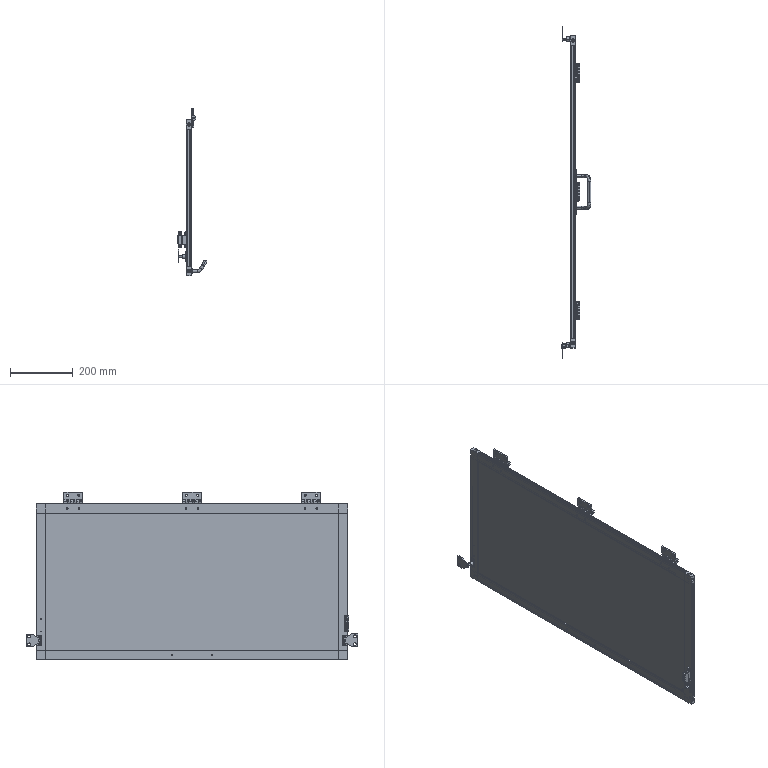Part | SolidWorks | 28 solids | 859 faces | box 95.2 x 1060 x 535 mm | volume 3524828 mm3 | plane 500 | cylinder 316 | cone 35 | torus 6 | spline 2 | commonest cylinder face diameters 5 x86 11 x56 7 x32 6.6 x24 2.5 x18 14.5 x18